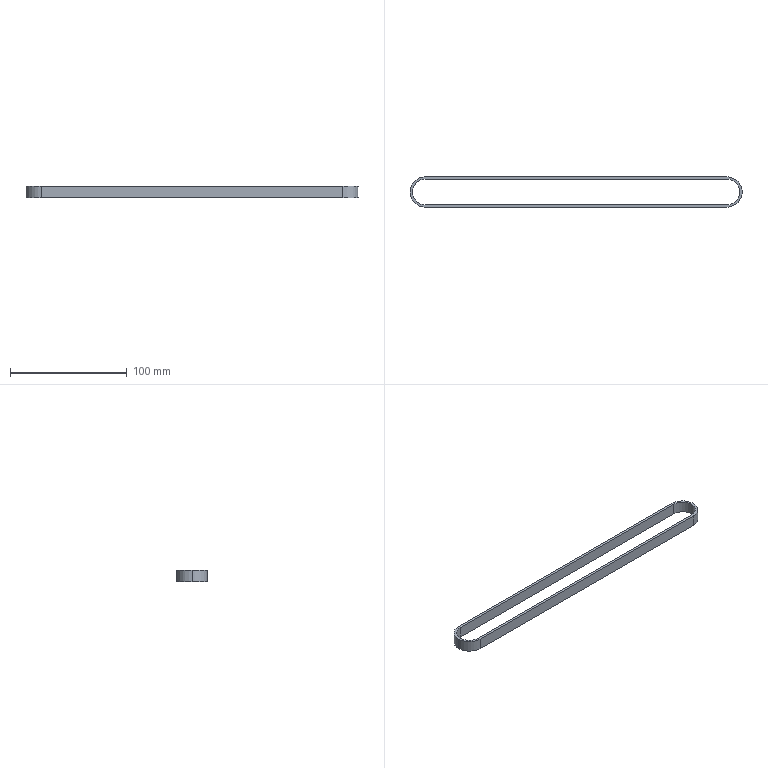Part | STEP file | HTBN540S3M-100 | 1 solid | 12 faces | box 284.5 x 26 x 10 mm | volume 11848 mm3 | cylinder 6 | plane 6 | commonest cylinder face diameters 22 x3 26 x3
STEP:
#1=CARTESIAN_POINT('',(0.,11.,5.));
#2=VERTEX_POINT('',#1);
#3=CARTESIAN_POINT('',(-11.,0.,5.));
#4=VERTEX_POINT('',#3);
#5=CARTESIAN_POINT('',(0.,0.,5.));
#6=DIRECTION('',(0.,0.,1.));
#7=DIRECTION('',(1.,0.,0.));
#8=AXIS2_PLACEMENT_3D('',#5,#6,#7);
#9=CIRCLE('',#8,11.);
#10=EDGE_CURVE('',#2,#4,#9,.T.);
#11=ORIENTED_EDGE('',*,*,#10,.T.);
#12=CARTESIAN_POINT('',(-11.,0.,-5.));
#13=VERTEX_POINT('',#12);
#14=CARTESIAN_POINT('',(-11.,0.,5.));
#15=DIRECTION('',(0.,0.,-1.));
#16=VECTOR('',#15,1000.);
#17=LINE('',#14,#16);
#18=EDGE_CURVE('',#4,#13,#17,.T.);
#19=ORIENTED_EDGE('',*,*,#18,.T.);
#20=CARTESIAN_POINT('',(0.,11.,-5.));
#21=VERTEX_POINT('',#20);
#22=CARTESIAN_POINT('',(0.,0.,-5.));
#23=DIRECTION('',(0.,0.,1.));
#24=DIRECTION('',(1.,0.,0.));
#25=AXIS2_PLACEMENT_3D('',#22,#23,#24);
#26=CIRCLE('',#25,11.);
#27=EDGE_CURVE('',#21,#13,#26,.T.);
#28=ORIENTED_EDGE('',*,*,#27,.F.);
#29=CARTESIAN_POINT('',(0.,11.,5.));
#30=DIRECTION('',(0.,0.,-1.));
#31=VECTOR('',#30,1000.);
#32=LINE('',#29,#31);
#33=EDGE_CURVE('',#2,#21,#32,.T.);
#34=ORIENTED_EDGE('',*,*,#33,.F.);
#35=EDGE_LOOP('',(#11,#19,#28,#34));
#36=FACE_OUTER_BOUND('',#35,.T.);
#37=CARTESIAN_POINT('',(0.,0.,5.));
#38=DIRECTION('',(0.,0.,-1.));
#39=DIRECTION('',(-1.,0.,0.));
#40=AXIS2_PLACEMENT_3D('',#37,#38,#39);
#41=CYLINDRICAL_SURFACE('',#40,11.);
#42=ADVANCED_FACE('',(#36),#41,.F.);
#43=CARTESIAN_POINT('',(-13.,0.,5.));
#44=VERTEX_POINT('',#43);
#45=CARTESIAN_POINT('',(0.,-13.,5.));
#46=VERTEX_POINT('',#45);
#47=CARTESIAN_POINT('',(0.,0.,5.));
#48=DIRECTION('',(0.,0.,1.));
#49=DIRECTION('',(1.,0.,0.));
#50=AXIS2_PLACEMENT_3D('',#47,#48,#49);
#51=CIRCLE('',#50,13.);
#52=EDGE_CURVE('',#44,#46,#51,.T.);
#53=ORIENTED_EDGE('',*,*,#52,.F.);
#54=CARTESIAN_POINT('',(-13.,0.,-5.));
#55=VERTEX_POINT('',#54);
#56=CARTESIAN_POINT('',(-13.,0.,5.));
#57=DIRECTION('',(0.,0.,-1.));
#58=VECTOR('',#57,1000.);
#59=LINE('',#56,#58);
#60=EDGE_CURVE('',#44,#55,#59,.T.);
#61=ORIENTED_EDGE('',*,*,#60,.T.);
#62=CARTESIAN_POINT('',(0.,-13.,-5.));
#63=VERTEX_POINT('',#62);
#64=CARTESIAN_POINT('',(0.,0.,-5.));
#65=DIRECTION('',(0.,0.,1.));
#66=DIRECTION('',(1.,0.,0.));
#67=AXIS2_PLACEMENT_3D('',#64,#65,#66);
#68=CIRCLE('',#67,13.);
#69=EDGE_CURVE('',#55,#63,#68,.T.);
#70=ORIENTED_EDGE('',*,*,#69,.T.);
#71=CARTESIAN_POINT('',(0.,-13.,5.));
#72=DIRECTION('',(0.,0.,-1.));
#73=VECTOR('',#72,1000.);
#74=LINE('',#71,#73);
#75=EDGE_CURVE('',#46,#63,#74,.T.);
#76=ORIENTED_EDGE('',*,*,#75,.F.);
#77=EDGE_LOOP('',(#53,#61,#70,#76));
#78=FACE_OUTER_BOUND('',#77,.T.);
#79=CARTESIAN_POINT('',(0.,0.,5.));
#80=DIRECTION('',(0.,0.,-1.));
#81=DIRECTION('',(-1.,0.,0.));
#82=AXIS2_PLACEMENT_3D('',#79,#80,#81);
#83=CYLINDRICAL_SURFACE('',#82,13.);
#84=ADVANCED_FACE('',(#78),#83,.T.);
#85=CARTESIAN_POINT('',(0.,13.,5.));
#86=VERTEX_POINT('',#85);
#87=CARTESIAN_POINT('',(0.,0.,5.));
#88=DIRECTION('',(0.,0.,1.));
#89=DIRECTION('',(1.,0.,0.));
#90=AXIS2_PLACEMENT_3D('',#87,#88,#89);
#91=CIRCLE('',#90,13.);
#92=EDGE_CURVE('',#86,#44,#91,.T.);
#93=ORIENTED_EDGE('',*,*,#92,.T.);
#94=ORIENTED_EDGE('',*,*,#52,.T.);
#95=CARTESIAN_POINT('',(258.5,-13.,5.));
#96=VERTEX_POINT('',#95);
#97=CARTESIAN_POINT('',(0.,-13.,5.));
#98=DIRECTION('',(1.,0.,0.));
#99=VECTOR('',#98,1000.);
#100=LINE('',#97,#99);
#101=EDGE_CURVE('',#46,#96,#100,.T.);
#102=ORIENTED_EDGE('',*,*,#101,.T.);
#103=CARTESIAN_POINT('',(258.5,13.,5.));
#104=VERTEX_POINT('',#103);
#105=CARTESIAN_POINT('',(258.5,0.,5.));
#106=DIRECTION('',(0.,0.,1.));
#107=DIRECTION('',(1.,0.,0.));
#108=AXIS2_PLACEMENT_3D('',#105,#106,#107);
#109=CIRCLE('',#108,13.);
#110=EDGE_CURVE('',#96,#104,#109,.T.);
#111=ORIENTED_EDGE('',*,*,#110,.T.);
#112=CARTESIAN_POINT('',(0.,13.,5.));
#113=DIRECTION('',(-1.,0.,0.));
#114=VECTOR('',#113,1000.);
#115=LINE('',#112,#114);
#116=EDGE_CURVE('',#104,#86,#115,.T.);
#117=ORIENTED_EDGE('',*,*,#116,.T.);
#118=EDGE_LOOP('',(#93,#94,#102,#111,#117));
#119=FACE_OUTER_BOUND('',#118,.T.);
#120=CARTESIAN_POINT('',(0.,-11.,5.));
#121=VERTEX_POINT('',#120);
#122=CARTESIAN_POINT('',(258.5,-11.,5.));
#123=VERTEX_POINT('',#122);
#124=CARTESIAN_POINT('',(0.,-11.,5.));
#125=DIRECTION('',(1.,0.,0.));
#126=VECTOR('',#125,1000.);
#127=LINE('',#124,#126);
#128=EDGE_CURVE('',#121,#123,#127,.T.);
#129=ORIENTED_EDGE('',*,*,#128,.F.);
#130=CARTESIAN_POINT('',(0.,0.,5.));
#131=DIRECTION('',(0.,0.,1.));
#132=DIRECTION('',(1.,0.,0.));
#133=AXIS2_PLACEMENT_3D('',#130,#131,#132);
#134=CIRCLE('',#133,11.);
#135=EDGE_CURVE('',#4,#121,#134,.T.);
#136=ORIENTED_EDGE('',*,*,#135,.F.);
#137=ORIENTED_EDGE('',*,*,#10,.F.);
#138=CARTESIAN_POINT('',(258.5,11.,5.));
#139=VERTEX_POINT('',#138);
#140=CARTESIAN_POINT('',(0.,11.,5.));
#141=DIRECTION('',(-1.,0.,0.));
#142=VECTOR('',#141,1000.);
#143=LINE('',#140,#142);
#144=EDGE_CURVE('',#139,#2,#143,.T.);
#145=ORIENTED_EDGE('',*,*,#144,.F.);
#146=CARTESIAN_POINT('',(258.5,0.,5.));
#147=DIRECTION('',(0.,0.,1.));
#148=DIRECTION('',(1.,0.,0.));
#149=AXIS2_PLACEMENT_3D('',#146,#147,#148);
#150=CIRCLE('',#149,11.);
#151=EDGE_CURVE('',#123,#139,#150,.T.);
#152=ORIENTED_EDGE('',*,*,#151,.F.);
#153=EDGE_LOOP('',(#129,#136,#137,#145,#152));
#154=FACE_BOUND('',#153,.T.);
#155=CARTESIAN_POINT('',(0.,0.,5.));
#156=DIRECTION('',(0.,0.,1.));
#157=DIRECTION('',(1.,0.,0.));
#158=AXIS2_PLACEMENT_3D('',#155,#156,#157);
#159=PLANE('',#158);
#160=ADVANCED_FACE('',(#119,#154),#159,.T.);
#161=CARTESIAN_POINT('',(0.,13.,-5.));
#162=VERTEX_POINT('',#161);
#163=CARTESIAN_POINT('',(0.,0.,-5.));
#164=DIRECTION('',(0.,0.,1.));
#165=DIRECTION('',(1.,0.,0.));
#166=AXIS2_PLACEMENT_3D('',#163,#164,#165);
#167=CIRCLE('',#166,13.);
#168=EDGE_CURVE('',#162,#55,#167,.T.);
#169=ORIENTED_EDGE('',*,*,#168,.F.);
#170=CARTESIAN_POINT('',(258.5,13.,-5.));
#171=VERTEX_POINT('',#170);
#172=CARTESIAN_POINT('',(0.,13.,-5.));
#173=DIRECTION('',(-1.,0.,0.));
#174=VECTOR('',#173,1000.);
#175=LINE('',#172,#174);
#176=EDGE_CURVE('',#171,#162,#175,.T.);
#177=ORIENTED_EDGE('',*,*,#176,.F.);
#178=CARTESIAN_POINT('',(258.5,-13.,-5.));
#179=VERTEX_POINT('',#178);
#180=CARTESIAN_POINT('',(258.5,0.,-5.));
#181=DIRECTION('',(0.,0.,1.));
#182=DIRECTION('',(1.,0.,0.));
#183=AXIS2_PLACEMENT_3D('',#180,#181,#182);
#184=CIRCLE('',#183,13.);
#185=EDGE_CURVE('',#179,#171,#184,.T.);
#186=ORIENTED_EDGE('',*,*,#185,.F.);
#187=CARTESIAN_POINT('',(0.,-13.,-5.));
#188=DIRECTION('',(1.,0.,0.));
#189=VECTOR('',#188,1000.);
#190=LINE('',#187,#189);
#191=EDGE_CURVE('',#63,#179,#190,.T.);
#192=ORIENTED_EDGE('',*,*,#191,.F.);
#193=ORIENTED_EDGE('',*,*,#69,.F.);
#194=EDGE_LOOP('',(#169,#177,#186,#192,#193));
#195=FACE_OUTER_BOUND('',#194,.T.);
#196=ORIENTED_EDGE('',*,*,#27,.T.);
#197=CARTESIAN_POINT('',(0.,-11.,-5.));
#198=VERTEX_POINT('',#197);
#199=CARTESIAN_POINT('',(0.,0.,-5.));
#200=DIRECTION('',(0.,0.,1.));
#201=DIRECTION('',(1.,0.,0.));
#202=AXIS2_PLACEMENT_3D('',#199,#200,#201);
#203=CIRCLE('',#202,11.);
#204=EDGE_CURVE('',#13,#198,#203,.T.);
#205=ORIENTED_EDGE('',*,*,#204,.T.);
#206=CARTESIAN_POINT('',(258.5,-11.,-5.));
#207=VERTEX_POINT('',#206);
#208=CARTESIAN_POINT('',(0.,-11.,-5.));
#209=DIRECTION('',(1.,0.,0.));
#210=VECTOR('',#209,1000.);
#211=LINE('',#208,#210);
#212=EDGE_CURVE('',#198,#207,#211,.T.);
#213=ORIENTED_EDGE('',*,*,#212,.T.);
#214=CARTESIAN_POINT('',(258.5,11.,-5.));
#215=VERTEX_POINT('',#214);
#216=CARTESIAN_POINT('',(258.5,0.,-5.));
#217=DIRECTION('',(0.,0.,1.));
#218=DIRECTION('',(1.,0.,0.));
#219=AXIS2_PLACEMENT_3D('',#216,#217,#218);
#220=CIRCLE('',#219,11.);
#221=EDGE_CURVE('',#207,#215,#220,.T.);
#222=ORIENTED_EDGE('',*,*,#221,.T.);
#223=CARTESIAN_POINT('',(0.,11.,-5.));
#224=DIRECTION('',(-1.,0.,0.));
#225=VECTOR('',#224,1000.);
#226=LINE('',#223,#225);
#227=EDGE_CURVE('',#215,#21,#226,.T.);
#228=ORIENTED_EDGE('',*,*,#227,.T.);
#229=EDGE_LOOP('',(#196,#205,#213,#222,#228));
#230=FACE_BOUND('',#229,.T.);
#231=CARTESIAN_POINT('',(0.,0.,-5.));
#232=DIRECTION('',(0.,0.,1.));
#233=DIRECTION('',(1.,0.,0.));
#234=AXIS2_PLACEMENT_3D('',#231,#232,#233);
#235=PLANE('',#234);
#236=ADVANCED_FACE('',(#195,#230),#235,.F.);
#237=ORIENTED_EDGE('',*,*,#60,.F.);
#238=ORIENTED_EDGE('',*,*,#92,.F.);
#239=CARTESIAN_POINT('',(0.,13.,5.));
#240=DIRECTION('',(0.,0.,-1.));
#241=VECTOR('',#240,1000.);
#242=LINE('',#239,#241);
#243=EDGE_CURVE('',#86,#162,#242,.T.);
#244=ORIENTED_EDGE('',*,*,#243,.T.);
#245=ORIENTED_EDGE('',*,*,#168,.T.);
#246=EDGE_LOOP('',(#237,#238,#244,#245));
#247=FACE_OUTER_BOUND('',#246,.T.);
#248=CARTESIAN_POINT('',(0.,0.,5.));
#249=DIRECTION('',(0.,0.,-1.));
#250=DIRECTION('',(-1.,0.,0.));
#251=AXIS2_PLACEMENT_3D('',#248,#249,#250);
#252=CYLINDRICAL_SURFACE('',#251,13.);
#253=ADVANCED_FACE('',(#247),#252,.T.);
#254=ORIENTED_EDGE('',*,*,#191,.T.);
#255=CARTESIAN_POINT('',(258.5,-13.,5.));
#256=DIRECTION('',(0.,0.,-1.));
#257=VECTOR('',#256,1000.);
#258=LINE('',#255,#257);
#259=EDGE_CURVE('',#96,#179,#258,.T.);
#260=ORIENTED_EDGE('',*,*,#259,.F.);
#261=ORIENTED_EDGE('',*,*,#101,.F.);
#262=ORIENTED_EDGE('',*,*,#75,.T.);
#263=EDGE_LOOP('',(#254,#260,#261,#262));
#264=FACE_OUTER_BOUND('',#263,.T.);
#265=CARTESIAN_POINT('',(0.,-13.,5.));
#266=DIRECTION('',(0.,1.,0.));
#267=DIRECTION('',(0.,0.,1.));
#268=AXIS2_PLACEMENT_3D('',#265,#266,#267);
#269=PLANE('',#268);
#270=ADVANCED_FACE('',(#264),#269,.F.);
#271=ORIENTED_EDGE('',*,*,#185,.T.);
#272=CARTESIAN_POINT('',(258.5,13.,5.));
#273=DIRECTION('',(0.,0.,-1.));
#274=VECTOR('',#273,1000.);
#275=LINE('',#272,#274);
#276=EDGE_CURVE('',#104,#171,#275,.T.);
#277=ORIENTED_EDGE('',*,*,#276,.F.);
#278=ORIENTED_EDGE('',*,*,#110,.F.);
#279=ORIENTED_EDGE('',*,*,#259,.T.);
#280=EDGE_LOOP('',(#271,#277,#278,#279));
#281=FACE_OUTER_BOUND('',#280,.T.);
#282=CARTESIAN_POINT('',(258.5,0.,5.));
#283=DIRECTION('',(0.,0.,-1.));
#284=DIRECTION('',(-1.,0.,0.));
#285=AXIS2_PLACEMENT_3D('',#282,#283,#284);
#286=CYLINDRICAL_SURFACE('',#285,13.);
#287=ADVANCED_FACE('',(#281),#286,.T.);
#288=ORIENTED_EDGE('',*,*,#176,.T.);
#289=ORIENTED_EDGE('',*,*,#243,.F.);
#290=ORIENTED_EDGE('',*,*,#116,.F.);
#291=ORIENTED_EDGE('',*,*,#276,.T.);
#292=EDGE_LOOP('',(#288,#289,#290,#291));
#293=FACE_OUTER_BOUND('',#292,.T.);
#294=CARTESIAN_POINT('',(0.,13.,5.));
#295=DIRECTION('',(0.,-1.,0.));
#296=DIRECTION('',(0.,0.,-1.));
#297=AXIS2_PLACEMENT_3D('',#294,#295,#296);
#298=PLANE('',#297);
#299=ADVANCED_FACE('',(#293),#298,.F.);
#300=ORIENTED_EDGE('',*,*,#18,.F.);
#301=ORIENTED_EDGE('',*,*,#135,.T.);
#302=CARTESIAN_POINT('',(0.,-11.,5.));
#303=DIRECTION('',(0.,0.,-1.));
#304=VECTOR('',#303,1000.);
#305=LINE('',#302,#304);
#306=EDGE_CURVE('',#121,#198,#305,.T.);
#307=ORIENTED_EDGE('',*,*,#306,.T.);
#308=ORIENTED_EDGE('',*,*,#204,.F.);
#309=EDGE_LOOP('',(#300,#301,#307,#308));
#310=FACE_OUTER_BOUND('',#309,.T.);
#311=CARTESIAN_POINT('',(0.,0.,5.));
#312=DIRECTION('',(0.,0.,-1.));
#313=DIRECTION('',(-1.,0.,0.));
#314=AXIS2_PLACEMENT_3D('',#311,#312,#313);
#315=CYLINDRICAL_SURFACE('',#314,11.);
#316=ADVANCED_FACE('',(#310),#315,.F.);
#317=ORIENTED_EDGE('',*,*,#212,.F.);
#318=ORIENTED_EDGE('',*,*,#306,.F.);
#319=ORIENTED_EDGE('',*,*,#128,.T.);
#320=CARTESIAN_POINT('',(258.5,-11.,5.));
#321=DIRECTION('',(0.,0.,-1.));
#322=VECTOR('',#321,1000.);
#323=LINE('',#320,#322);
#324=EDGE_CURVE('',#123,#207,#323,.T.);
#325=ORIENTED_EDGE('',*,*,#324,.T.);
#326=EDGE_LOOP('',(#317,#318,#319,#325));
#327=FACE_OUTER_BOUND('',#326,.T.);
#328=CARTESIAN_POINT('',(0.,-11.,5.));
#329=DIRECTION('',(0.,1.,0.));
#330=DIRECTION('',(0.,0.,1.));
#331=AXIS2_PLACEMENT_3D('',#328,#329,#330);
#332=PLANE('',#331);
#333=ADVANCED_FACE('',(#327),#332,.T.);
#334=ORIENTED_EDGE('',*,*,#221,.F.);
#335=ORIENTED_EDGE('',*,*,#324,.F.);
#336=ORIENTED_EDGE('',*,*,#151,.T.);
#337=CARTESIAN_POINT('',(258.5,11.,5.));
#338=DIRECTION('',(0.,0.,-1.));
#339=VECTOR('',#338,1000.);
#340=LINE('',#337,#339);
#341=EDGE_CURVE('',#139,#215,#340,.T.);
#342=ORIENTED_EDGE('',*,*,#341,.T.);
#343=EDGE_LOOP('',(#334,#335,#336,#342));
#344=FACE_OUTER_BOUND('',#343,.T.);
#345=CARTESIAN_POINT('',(258.5,0.,5.));
#346=DIRECTION('',(0.,0.,-1.));
#347=DIRECTION('',(-1.,0.,0.));
#348=AXIS2_PLACEMENT_3D('',#345,#346,#347);
#349=CYLINDRICAL_SURFACE('',#348,11.);
#350=ADVANCED_FACE('',(#344),#349,.F.);
#351=ORIENTED_EDGE('',*,*,#227,.F.);
#352=ORIENTED_EDGE('',*,*,#341,.F.);
#353=ORIENTED_EDGE('',*,*,#144,.T.);
#354=ORIENTED_EDGE('',*,*,#33,.T.);
#355=EDGE_LOOP('',(#351,#352,#353,#354));
#356=FACE_OUTER_BOUND('',#355,.T.);
#357=CARTESIAN_POINT('',(0.,11.,5.));
#358=DIRECTION('',(0.,-1.,0.));
#359=DIRECTION('',(0.,0.,-1.));
#360=AXIS2_PLACEMENT_3D('',#357,#358,#359);
#361=PLANE('',#360);
#362=ADVANCED_FACE('',(#356),#361,.T.);
#363=CLOSED_SHELL('',(#42,#84,#160,#236,#253,#270,#287,#299,#316,#333,#350,#362));
#364=MANIFOLD_SOLID_BREP('',#363);
#365=CARTESIAN_POINT('',(0.,0.,0.));
#366=DIRECTION('',(0.,0.,1.));
#367=DIRECTION('',(1.,0.,0.));
#368=AXIS2_PLACEMENT_3D('',#365,#366,#367);
#369=(LENGTH_UNIT()NAMED_UNIT(*)SI_UNIT(.MILLI.,.METRE.));
#370=UNCERTAINTY_MEASURE_WITH_UNIT(LENGTH_MEASURE(0.00001),#369,'','');
#371=(NAMED_UNIT(*)PLANE_ANGLE_UNIT()SI_UNIT($,.RADIAN.));
#372=(NAMED_UNIT(*)SI_UNIT($,.STERADIAN.)SOLID_ANGLE_UNIT());
#373=(GEOMETRIC_REPRESENTATION_CONTEXT(3)GLOBAL_UNCERTAINTY_ASSIGNED_CONTEXT((#370))GLOBAL_UNIT_ASSIGNED_CONTEXT((#369,#371,#372))REPRESENTATION_CONTEXT('',''));
#374=ADVANCED_BREP_SHAPE_REPRESENTATION('',(#364,#368),#373);